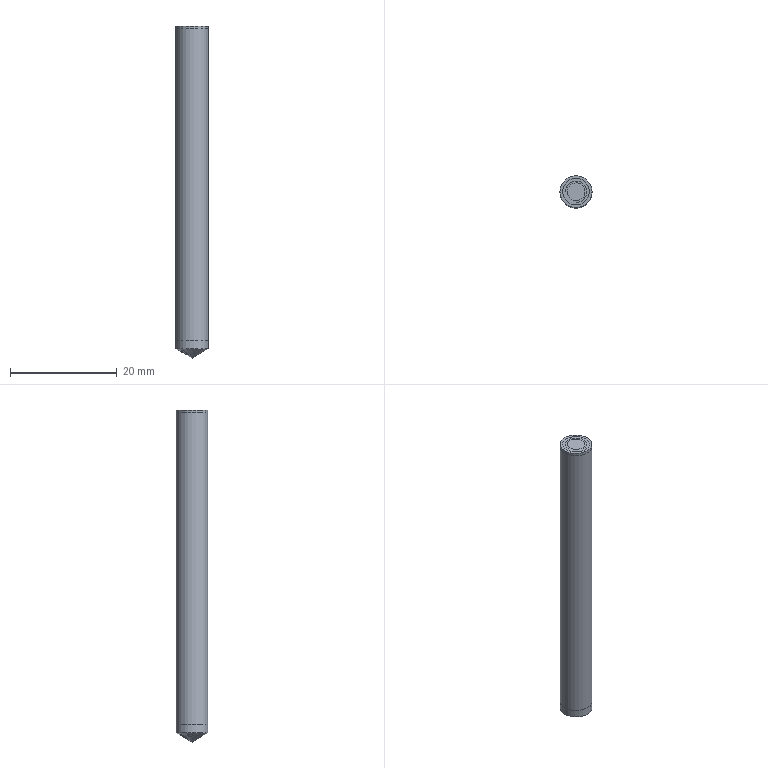Part | STEP file | EE030606000 | 2 solids | 45 faces | box 6 x 6 x 62.232 mm | volume 3333 mm3 | plane 15 | other 13 | cone 11 | cylinder 5 | torus 1 | commonest cylinder face diameters 6 x2 3.333 x1 3.987 x1 4 x1